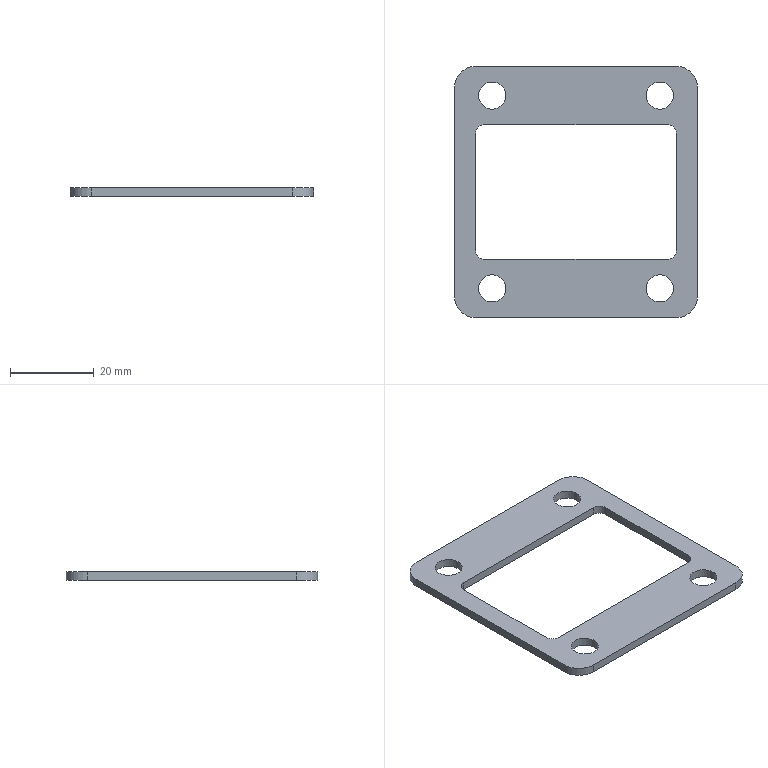Part | NX | features BREP 1 | 1 solid | 22 faces | box 58 x 60 x 2 mm | volume 3586 mm3 | cylinder 12 | plane 10 | commonest cylinder face diameters 4 x4 6.5 x4 10 x4
STEP:
#1=CARTESIAN_POINT('',(-23.25,23.,2.));
#2=VERTEX_POINT('',#1);
#3=CARTESIAN_POINT('',(-20.,23.,2.));
#4=DIRECTION('',(0.,0.,1.));
#5=DIRECTION('',(-1.,0.,0.));
#6=AXIS2_PLACEMENT_3D('',#3,#4,#5);
#7=CIRCLE('',#6,3.25);
#8=EDGE_CURVE('',#2,#2,#7,.T.);
#9=ORIENTED_EDGE('',*,*,#8,.T.);
#10=EDGE_LOOP('',(#9));
#11=FACE_BOUND('',#10,.T.);
#12=CARTESIAN_POINT('',(-23.25,23.,0.));
#13=VERTEX_POINT('',#12);
#14=CARTESIAN_POINT('',(-20.,23.,0.));
#15=DIRECTION('',(0.,0.,1.));
#16=DIRECTION('',(-1.,0.,0.));
#17=AXIS2_PLACEMENT_3D('',#14,#15,#16);
#18=CIRCLE('',#17,3.25);
#19=EDGE_CURVE('',#13,#13,#18,.T.);
#20=ORIENTED_EDGE('',*,*,#19,.F.);
#21=EDGE_LOOP('',(#20));
#22=FACE_BOUND('',#21,.T.);
#23=CARTESIAN_POINT('',(-20.,23.,0.));
#24=DIRECTION('',(0.,0.,1.));
#25=DIRECTION('',(1.,0.,0.));
#26=AXIS2_PLACEMENT_3D('',#23,#24,#25);
#27=CYLINDRICAL_SURFACE('',#26,3.25);
#28=ADVANCED_FACE('',(#11,#22),#27,.F.);
#29=CARTESIAN_POINT('',(-16.75,-23.,2.));
#30=VERTEX_POINT('',#29);
#31=CARTESIAN_POINT('',(-20.,-23.,2.));
#32=DIRECTION('',(0.,0.,1.));
#33=DIRECTION('',(1.,0.,0.));
#34=AXIS2_PLACEMENT_3D('',#31,#32,#33);
#35=CIRCLE('',#34,3.25);
#36=EDGE_CURVE('',#30,#30,#35,.T.);
#37=ORIENTED_EDGE('',*,*,#36,.T.);
#38=EDGE_LOOP('',(#37));
#39=FACE_BOUND('',#38,.T.);
#40=CARTESIAN_POINT('',(-16.75,-23.,0.));
#41=VERTEX_POINT('',#40);
#42=CARTESIAN_POINT('',(-20.,-23.,0.));
#43=DIRECTION('',(0.,0.,1.));
#44=DIRECTION('',(1.,0.,0.));
#45=AXIS2_PLACEMENT_3D('',#42,#43,#44);
#46=CIRCLE('',#45,3.25);
#47=EDGE_CURVE('',#41,#41,#46,.T.);
#48=ORIENTED_EDGE('',*,*,#47,.F.);
#49=EDGE_LOOP('',(#48));
#50=FACE_BOUND('',#49,.T.);
#51=CARTESIAN_POINT('',(-20.,-23.,0.));
#52=DIRECTION('',(0.,0.,1.));
#53=DIRECTION('',(1.,0.,0.));
#54=AXIS2_PLACEMENT_3D('',#51,#52,#53);
#55=CYLINDRICAL_SURFACE('',#54,3.25);
#56=ADVANCED_FACE('',(#39,#50),#55,.F.);
#57=CARTESIAN_POINT('',(16.75,-23.,2.));
#58=VERTEX_POINT('',#57);
#59=CARTESIAN_POINT('',(20.,-23.,2.));
#60=DIRECTION('',(0.,0.,1.));
#61=DIRECTION('',(-1.,0.,0.));
#62=AXIS2_PLACEMENT_3D('',#59,#60,#61);
#63=CIRCLE('',#62,3.25);
#64=EDGE_CURVE('',#58,#58,#63,.T.);
#65=ORIENTED_EDGE('',*,*,#64,.T.);
#66=EDGE_LOOP('',(#65));
#67=FACE_BOUND('',#66,.T.);
#68=CARTESIAN_POINT('',(16.75,-23.,0.));
#69=VERTEX_POINT('',#68);
#70=CARTESIAN_POINT('',(20.,-23.,0.));
#71=DIRECTION('',(0.,0.,1.));
#72=DIRECTION('',(-1.,0.,0.));
#73=AXIS2_PLACEMENT_3D('',#70,#71,#72);
#74=CIRCLE('',#73,3.25);
#75=EDGE_CURVE('',#69,#69,#74,.T.);
#76=ORIENTED_EDGE('',*,*,#75,.F.);
#77=EDGE_LOOP('',(#76));
#78=FACE_BOUND('',#77,.T.);
#79=CARTESIAN_POINT('',(20.,-23.,0.));
#80=DIRECTION('',(0.,0.,1.));
#81=DIRECTION('',(1.,0.,0.));
#82=AXIS2_PLACEMENT_3D('',#79,#80,#81);
#83=CYLINDRICAL_SURFACE('',#82,3.25);
#84=ADVANCED_FACE('',(#67,#78),#83,.F.);
#85=CARTESIAN_POINT('',(23.25,23.,2.));
#86=VERTEX_POINT('',#85);
#87=CARTESIAN_POINT('',(20.,23.,2.));
#88=DIRECTION('',(0.,0.,1.));
#89=DIRECTION('',(1.,0.,0.));
#90=AXIS2_PLACEMENT_3D('',#87,#88,#89);
#91=CIRCLE('',#90,3.25);
#92=EDGE_CURVE('',#86,#86,#91,.T.);
#93=ORIENTED_EDGE('',*,*,#92,.T.);
#94=EDGE_LOOP('',(#93));
#95=FACE_BOUND('',#94,.T.);
#96=CARTESIAN_POINT('',(23.25,23.,0.));
#97=VERTEX_POINT('',#96);
#98=CARTESIAN_POINT('',(20.,23.,0.));
#99=DIRECTION('',(0.,0.,1.));
#100=DIRECTION('',(1.,0.,0.));
#101=AXIS2_PLACEMENT_3D('',#98,#99,#100);
#102=CIRCLE('',#101,3.25);
#103=EDGE_CURVE('',#97,#97,#102,.T.);
#104=ORIENTED_EDGE('',*,*,#103,.F.);
#105=EDGE_LOOP('',(#104));
#106=FACE_BOUND('',#105,.T.);
#107=CARTESIAN_POINT('',(20.,23.,0.));
#108=DIRECTION('',(0.,0.,1.));
#109=DIRECTION('',(1.,0.,0.));
#110=AXIS2_PLACEMENT_3D('',#107,#108,#109);
#111=CYLINDRICAL_SURFACE('',#110,3.25);
#112=ADVANCED_FACE('',(#95,#106),#111,.F.);
#113=ORIENTED_EDGE('',*,*,#8,.F.);
#114=EDGE_LOOP('',(#113));
#115=FACE_BOUND('',#114,.T.);
#116=ORIENTED_EDGE('',*,*,#36,.F.);
#117=EDGE_LOOP('',(#116));
#118=FACE_BOUND('',#117,.T.);
#119=ORIENTED_EDGE('',*,*,#64,.F.);
#120=EDGE_LOOP('',(#119));
#121=FACE_BOUND('',#120,.T.);
#122=ORIENTED_EDGE('',*,*,#92,.F.);
#123=EDGE_LOOP('',(#122));
#124=FACE_BOUND('',#123,.T.);
#125=CARTESIAN_POINT('',(-29.,25.,2.));
#126=VERTEX_POINT('',#125);
#127=CARTESIAN_POINT('',(-29.,-25.,2.));
#128=VERTEX_POINT('',#127);
#129=CARTESIAN_POINT('',(-29.,30.,2.));
#130=DIRECTION('',(0.,-1.,0.));
#131=VECTOR('',#130,1000.);
#132=LINE('',#129,#131);
#133=EDGE_CURVE('',#126,#128,#132,.T.);
#134=ORIENTED_EDGE('',*,*,#133,.T.);
#135=CARTESIAN_POINT('',(-24.,-30.,2.));
#136=VERTEX_POINT('',#135);
#137=CARTESIAN_POINT('',(-24.,-25.,2.));
#138=DIRECTION('',(0.,0.,1.));
#139=DIRECTION('',(1.,0.,0.));
#140=AXIS2_PLACEMENT_3D('',#137,#138,#139);
#141=CIRCLE('',#140,5.);
#142=EDGE_CURVE('',#128,#136,#141,.T.);
#143=ORIENTED_EDGE('',*,*,#142,.T.);
#144=CARTESIAN_POINT('',(24.,-30.,2.));
#145=VERTEX_POINT('',#144);
#146=CARTESIAN_POINT('',(-29.,-30.,2.));
#147=DIRECTION('',(1.,0.,0.));
#148=VECTOR('',#147,1000.);
#149=LINE('',#146,#148);
#150=EDGE_CURVE('',#136,#145,#149,.T.);
#151=ORIENTED_EDGE('',*,*,#150,.T.);
#152=CARTESIAN_POINT('',(29.,-25.,2.));
#153=VERTEX_POINT('',#152);
#154=CARTESIAN_POINT('',(24.,-25.,2.));
#155=DIRECTION('',(0.,0.,1.));
#156=DIRECTION('',(1.,0.,0.));
#157=AXIS2_PLACEMENT_3D('',#154,#155,#156);
#158=CIRCLE('',#157,5.);
#159=EDGE_CURVE('',#145,#153,#158,.T.);
#160=ORIENTED_EDGE('',*,*,#159,.T.);
#161=CARTESIAN_POINT('',(29.,25.,2.));
#162=VERTEX_POINT('',#161);
#163=CARTESIAN_POINT('',(29.,30.,2.));
#164=DIRECTION('',(0.,1.,0.));
#165=VECTOR('',#164,1000.);
#166=LINE('',#163,#165);
#167=EDGE_CURVE('',#153,#162,#166,.T.);
#168=ORIENTED_EDGE('',*,*,#167,.T.);
#169=CARTESIAN_POINT('',(24.,30.,2.));
#170=VERTEX_POINT('',#169);
#171=CARTESIAN_POINT('',(24.,25.,2.));
#172=DIRECTION('',(0.,0.,1.));
#173=DIRECTION('',(1.,0.,0.));
#174=AXIS2_PLACEMENT_3D('',#171,#172,#173);
#175=CIRCLE('',#174,5.);
#176=EDGE_CURVE('',#162,#170,#175,.T.);
#177=ORIENTED_EDGE('',*,*,#176,.T.);
#178=CARTESIAN_POINT('',(-24.,30.,2.));
#179=VERTEX_POINT('',#178);
#180=CARTESIAN_POINT('',(-29.,30.,2.));
#181=DIRECTION('',(-1.,0.,0.));
#182=VECTOR('',#181,1000.);
#183=LINE('',#180,#182);
#184=EDGE_CURVE('',#170,#179,#183,.T.);
#185=ORIENTED_EDGE('',*,*,#184,.T.);
#186=CARTESIAN_POINT('',(-24.,25.,2.));
#187=DIRECTION('',(0.,0.,1.));
#188=DIRECTION('',(1.,0.,0.));
#189=AXIS2_PLACEMENT_3D('',#186,#187,#188);
#190=CIRCLE('',#189,5.);
#191=EDGE_CURVE('',#179,#126,#190,.T.);
#192=ORIENTED_EDGE('',*,*,#191,.T.);
#193=EDGE_LOOP('',(#134,#143,#151,#160,#168,#177,#185,#192));
#194=FACE_BOUND('',#193,.T.);
#195=CARTESIAN_POINT('',(22.,16.,2.));
#196=VERTEX_POINT('',#195);
#197=CARTESIAN_POINT('',(-22.,16.,2.));
#198=VERTEX_POINT('',#197);
#199=CARTESIAN_POINT('',(-24.,16.,2.));
#200=DIRECTION('',(-1.,0.,0.));
#201=VECTOR('',#200,1000.);
#202=LINE('',#199,#201);
#203=EDGE_CURVE('',#196,#198,#202,.T.);
#204=ORIENTED_EDGE('',*,*,#203,.F.);
#205=CARTESIAN_POINT('',(24.,14.,2.));
#206=VERTEX_POINT('',#205);
#207=CARTESIAN_POINT('',(22.,14.,2.));
#208=DIRECTION('',(0.,0.,-1.));
#209=DIRECTION('',(1.,0.,0.));
#210=AXIS2_PLACEMENT_3D('',#207,#208,#209);
#211=CIRCLE('',#210,2.);
#212=EDGE_CURVE('',#196,#206,#211,.T.);
#213=ORIENTED_EDGE('',*,*,#212,.T.);
#214=CARTESIAN_POINT('',(24.,-14.,2.));
#215=VERTEX_POINT('',#214);
#216=CARTESIAN_POINT('',(24.,16.,2.));
#217=DIRECTION('',(0.,1.,0.));
#218=VECTOR('',#217,1000.);
#219=LINE('',#216,#218);
#220=EDGE_CURVE('',#215,#206,#219,.T.);
#221=ORIENTED_EDGE('',*,*,#220,.F.);
#222=CARTESIAN_POINT('',(22.,-16.,2.));
#223=VERTEX_POINT('',#222);
#224=CARTESIAN_POINT('',(22.,-14.,2.));
#225=DIRECTION('',(0.,0.,-1.));
#226=DIRECTION('',(1.,0.,0.));
#227=AXIS2_PLACEMENT_3D('',#224,#225,#226);
#228=CIRCLE('',#227,2.);
#229=EDGE_CURVE('',#215,#223,#228,.T.);
#230=ORIENTED_EDGE('',*,*,#229,.T.);
#231=CARTESIAN_POINT('',(-22.,-16.,2.));
#232=VERTEX_POINT('',#231);
#233=CARTESIAN_POINT('',(-24.,-16.,2.));
#234=DIRECTION('',(1.,0.,0.));
#235=VECTOR('',#234,1000.);
#236=LINE('',#233,#235);
#237=EDGE_CURVE('',#232,#223,#236,.T.);
#238=ORIENTED_EDGE('',*,*,#237,.F.);
#239=CARTESIAN_POINT('',(-24.,-14.,2.));
#240=VERTEX_POINT('',#239);
#241=CARTESIAN_POINT('',(-22.,-14.,2.));
#242=DIRECTION('',(0.,0.,-1.));
#243=DIRECTION('',(1.,0.,0.));
#244=AXIS2_PLACEMENT_3D('',#241,#242,#243);
#245=CIRCLE('',#244,2.);
#246=EDGE_CURVE('',#232,#240,#245,.T.);
#247=ORIENTED_EDGE('',*,*,#246,.T.);
#248=CARTESIAN_POINT('',(-24.,14.,2.));
#249=VERTEX_POINT('',#248);
#250=CARTESIAN_POINT('',(-24.,16.,2.));
#251=DIRECTION('',(0.,-1.,0.));
#252=VECTOR('',#251,1000.);
#253=LINE('',#250,#252);
#254=EDGE_CURVE('',#249,#240,#253,.T.);
#255=ORIENTED_EDGE('',*,*,#254,.F.);
#256=CARTESIAN_POINT('',(-22.,14.,2.));
#257=DIRECTION('',(0.,0.,-1.));
#258=DIRECTION('',(1.,0.,0.));
#259=AXIS2_PLACEMENT_3D('',#256,#257,#258);
#260=CIRCLE('',#259,2.);
#261=EDGE_CURVE('',#249,#198,#260,.T.);
#262=ORIENTED_EDGE('',*,*,#261,.T.);
#263=EDGE_LOOP('',(#204,#213,#221,#230,#238,#247,#255,#262));
#264=FACE_BOUND('',#263,.T.);
#265=CARTESIAN_POINT('',(0.,0.,2.));
#266=DIRECTION('',(0.,0.,1.));
#267=DIRECTION('',(1.,0.,0.));
#268=AXIS2_PLACEMENT_3D('',#265,#266,#267);
#269=PLANE('',#268);
#270=ADVANCED_FACE('',(#115,#118,#121,#124,#194,#264),#269,.T.);
#271=ORIENTED_EDGE('',*,*,#19,.T.);
#272=EDGE_LOOP('',(#271));
#273=FACE_BOUND('',#272,.T.);
#274=ORIENTED_EDGE('',*,*,#47,.T.);
#275=EDGE_LOOP('',(#274));
#276=FACE_BOUND('',#275,.T.);
#277=ORIENTED_EDGE('',*,*,#75,.T.);
#278=EDGE_LOOP('',(#277));
#279=FACE_BOUND('',#278,.T.);
#280=ORIENTED_EDGE('',*,*,#103,.T.);
#281=EDGE_LOOP('',(#280));
#282=FACE_BOUND('',#281,.T.);
#283=CARTESIAN_POINT('',(-24.,-30.,0.));
#284=VERTEX_POINT('',#283);
#285=CARTESIAN_POINT('',(24.,-30.,0.));
#286=VERTEX_POINT('',#285);
#287=CARTESIAN_POINT('',(-29.,-30.,0.));
#288=DIRECTION('',(1.,0.,0.));
#289=VECTOR('',#288,1000.);
#290=LINE('',#287,#289);
#291=EDGE_CURVE('',#284,#286,#290,.T.);
#292=ORIENTED_EDGE('',*,*,#291,.F.);
#293=CARTESIAN_POINT('',(-29.,-25.,0.));
#294=VERTEX_POINT('',#293);
#295=CARTESIAN_POINT('',(-24.,-25.,0.));
#296=DIRECTION('',(0.,0.,-1.));
#297=DIRECTION('',(1.,0.,0.));
#298=AXIS2_PLACEMENT_3D('',#295,#296,#297);
#299=CIRCLE('',#298,5.);
#300=EDGE_CURVE('',#284,#294,#299,.T.);
#301=ORIENTED_EDGE('',*,*,#300,.T.);
#302=CARTESIAN_POINT('',(-29.,25.,0.));
#303=VERTEX_POINT('',#302);
#304=CARTESIAN_POINT('',(-29.,30.,0.));
#305=DIRECTION('',(0.,-1.,0.));
#306=VECTOR('',#305,1000.);
#307=LINE('',#304,#306);
#308=EDGE_CURVE('',#303,#294,#307,.T.);
#309=ORIENTED_EDGE('',*,*,#308,.F.);
#310=CARTESIAN_POINT('',(-24.,30.,0.));
#311=VERTEX_POINT('',#310);
#312=CARTESIAN_POINT('',(-24.,25.,0.));
#313=DIRECTION('',(0.,0.,-1.));
#314=DIRECTION('',(1.,0.,0.));
#315=AXIS2_PLACEMENT_3D('',#312,#313,#314);
#316=CIRCLE('',#315,5.);
#317=EDGE_CURVE('',#303,#311,#316,.T.);
#318=ORIENTED_EDGE('',*,*,#317,.T.);
#319=CARTESIAN_POINT('',(24.,30.,0.));
#320=VERTEX_POINT('',#319);
#321=CARTESIAN_POINT('',(-29.,30.,0.));
#322=DIRECTION('',(-1.,0.,0.));
#323=VECTOR('',#322,1000.);
#324=LINE('',#321,#323);
#325=EDGE_CURVE('',#320,#311,#324,.T.);
#326=ORIENTED_EDGE('',*,*,#325,.F.);
#327=CARTESIAN_POINT('',(29.,25.,0.));
#328=VERTEX_POINT('',#327);
#329=CARTESIAN_POINT('',(24.,25.,0.));
#330=DIRECTION('',(0.,0.,-1.));
#331=DIRECTION('',(1.,0.,0.));
#332=AXIS2_PLACEMENT_3D('',#329,#330,#331);
#333=CIRCLE('',#332,5.);
#334=EDGE_CURVE('',#320,#328,#333,.T.);
#335=ORIENTED_EDGE('',*,*,#334,.T.);
#336=CARTESIAN_POINT('',(29.,-25.,0.));
#337=VERTEX_POINT('',#336);
#338=CARTESIAN_POINT('',(29.,30.,0.));
#339=DIRECTION('',(0.,1.,0.));
#340=VECTOR('',#339,1000.);
#341=LINE('',#338,#340);
#342=EDGE_CURVE('',#337,#328,#341,.T.);
#343=ORIENTED_EDGE('',*,*,#342,.F.);
#344=CARTESIAN_POINT('',(24.,-25.,0.));
#345=DIRECTION('',(0.,0.,-1.));
#346=DIRECTION('',(1.,0.,0.));
#347=AXIS2_PLACEMENT_3D('',#344,#345,#346);
#348=CIRCLE('',#347,5.);
#349=EDGE_CURVE('',#337,#286,#348,.T.);
#350=ORIENTED_EDGE('',*,*,#349,.T.);
#351=EDGE_LOOP('',(#292,#301,#309,#318,#326,#335,#343,#350));
#352=FACE_BOUND('',#351,.T.);
#353=CARTESIAN_POINT('',(-22.,-16.,0.));
#354=VERTEX_POINT('',#353);
#355=CARTESIAN_POINT('',(22.,-16.,0.));
#356=VERTEX_POINT('',#355);
#357=CARTESIAN_POINT('',(-24.,-16.,0.));
#358=DIRECTION('',(1.,0.,0.));
#359=VECTOR('',#358,1000.);
#360=LINE('',#357,#359);
#361=EDGE_CURVE('',#354,#356,#360,.T.);
#362=ORIENTED_EDGE('',*,*,#361,.T.);
#363=CARTESIAN_POINT('',(24.,-14.,0.));
#364=VERTEX_POINT('',#363);
#365=CARTESIAN_POINT('',(22.,-14.,0.));
#366=DIRECTION('',(0.,0.,1.));
#367=DIRECTION('',(1.,0.,0.));
#368=AXIS2_PLACEMENT_3D('',#365,#366,#367);
#369=CIRCLE('',#368,2.);
#370=EDGE_CURVE('',#356,#364,#369,.T.);
#371=ORIENTED_EDGE('',*,*,#370,.T.);
#372=CARTESIAN_POINT('',(24.,14.,0.));
#373=VERTEX_POINT('',#372);
#374=CARTESIAN_POINT('',(24.,16.,0.));
#375=DIRECTION('',(0.,1.,0.));
#376=VECTOR('',#375,1000.);
#377=LINE('',#374,#376);
#378=EDGE_CURVE('',#364,#373,#377,.T.);
#379=ORIENTED_EDGE('',*,*,#378,.T.);
#380=CARTESIAN_POINT('',(22.,16.,0.));
#381=VERTEX_POINT('',#380);
#382=CARTESIAN_POINT('',(22.,14.,0.));
#383=DIRECTION('',(0.,0.,1.));
#384=DIRECTION('',(1.,0.,0.));
#385=AXIS2_PLACEMENT_3D('',#382,#383,#384);
#386=CIRCLE('',#385,2.);
#387=EDGE_CURVE('',#373,#381,#386,.T.);
#388=ORIENTED_EDGE('',*,*,#387,.T.);
#389=CARTESIAN_POINT('',(-22.,16.,0.));
#390=VERTEX_POINT('',#389);
#391=CARTESIAN_POINT('',(-24.,16.,0.));
#392=DIRECTION('',(-1.,0.,0.));
#393=VECTOR('',#392,1000.);
#394=LINE('',#391,#393);
#395=EDGE_CURVE('',#381,#390,#394,.T.);
#396=ORIENTED_EDGE('',*,*,#395,.T.);
#397=CARTESIAN_POINT('',(-24.,14.,0.));
#398=VERTEX_POINT('',#397);
#399=CARTESIAN_POINT('',(-22.,14.,0.));
#400=DIRECTION('',(0.,0.,1.));
#401=DIRECTION('',(1.,0.,0.));
#402=AXIS2_PLACEMENT_3D('',#399,#400,#401);
#403=CIRCLE('',#402,2.);
#404=EDGE_CURVE('',#390,#398,#403,.T.);
#405=ORIENTED_EDGE('',*,*,#404,.T.);
#406=CARTESIAN_POINT('',(-24.,-14.,0.));
#407=VERTEX_POINT('',#406);
#408=CARTESIAN_POINT('',(-24.,16.,0.));
#409=DIRECTION('',(0.,-1.,0.));
#410=VECTOR('',#409,1000.);
#411=LINE('',#408,#410);
#412=EDGE_CURVE('',#398,#407,#411,.T.);
#413=ORIENTED_EDGE('',*,*,#412,.T.);
#414=CARTESIAN_POINT('',(-22.,-14.,0.));
#415=DIRECTION('',(0.,0.,1.));
#416=DIRECTION('',(1.,0.,0.));
#417=AXIS2_PLACEMENT_3D('',#414,#415,#416);
#418=CIRCLE('',#417,2.);
#419=EDGE_CURVE('',#407,#354,#418,.T.);
#420=ORIENTED_EDGE('',*,*,#419,.T.);
#421=EDGE_LOOP('',(#362,#371,#379,#388,#396,#405,#413,#420));
#422=FACE_BOUND('',#421,.T.);
#423=CARTESIAN_POINT('',(0.,0.,0.));
#424=DIRECTION('',(0.,0.,1.));
#425=DIRECTION('',(1.,0.,0.));
#426=AXIS2_PLACEMENT_3D('',#423,#424,#425);
#427=PLANE('',#426);
#428=ADVANCED_FACE('',(#273,#276,#279,#282,#352,#422),#427,.F.);
#429=ORIENTED_EDGE('',*,*,#167,.F.);
#430=CARTESIAN_POINT('',(29.,-25.,2.));
#431=DIRECTION('',(0.,0.,-1.));
#432=VECTOR('',#431,1000.);
#433=LINE('',#430,#432);
#434=EDGE_CURVE('',#153,#337,#433,.T.);
#435=ORIENTED_EDGE('',*,*,#434,.T.);
#436=ORIENTED_EDGE('',*,*,#342,.T.);
#437=CARTESIAN_POINT('',(29.,25.,2.));
#438=DIRECTION('',(0.,0.,1.));
#439=VECTOR('',#438,1000.);
#440=LINE('',#437,#439);
#441=EDGE_CURVE('',#328,#162,#440,.T.);
#442=ORIENTED_EDGE('',*,*,#441,.T.);
#443=EDGE_LOOP('',(#429,#435,#436,#442));
#444=FACE_BOUND('',#443,.T.);
#445=CARTESIAN_POINT('',(29.,30.,2.));
#446=DIRECTION('',(-1.,0.,0.));
#447=DIRECTION('',(0.,-1.,0.));
#448=AXIS2_PLACEMENT_3D('',#445,#446,#447);
#449=PLANE('',#448);
#450=ADVANCED_FACE('',(#444),#449,.F.);
#451=ORIENTED_EDGE('',*,*,#184,.F.);
#452=CARTESIAN_POINT('',(24.,30.,2.));
#453=DIRECTION('',(0.,0.,-1.));
#454=VECTOR('',#453,1000.);
#455=LINE('',#452,#454);
#456=EDGE_CURVE('',#170,#320,#455,.T.);
#457=ORIENTED_EDGE('',*,*,#456,.T.);
#458=ORIENTED_EDGE('',*,*,#325,.T.);
#459=CARTESIAN_POINT('',(-24.,30.,2.));
#460=DIRECTION('',(0.,0.,1.));
#461=VECTOR('',#460,1000.);
#462=LINE('',#459,#461);
#463=EDGE_CURVE('',#311,#179,#462,.T.);
#464=ORIENTED_EDGE('',*,*,#463,.T.);
#465=EDGE_LOOP('',(#451,#457,#458,#464));
#466=FACE_BOUND('',#465,.T.);
#467=CARTESIAN_POINT('',(-29.,30.,2.));
#468=DIRECTION('',(0.,-1.,0.));
#469=DIRECTION('',(0.,0.,-1.));
#470=AXIS2_PLACEMENT_3D('',#467,#468,#469);
#471=PLANE('',#470);
#472=ADVANCED_FACE('',(#466),#471,.F.);
#473=ORIENTED_EDGE('',*,*,#308,.T.);
#474=CARTESIAN_POINT('',(-29.,-25.,2.));
#475=DIRECTION('',(0.,0.,1.));
#476=VECTOR('',#475,1000.);
#477=LINE('',#474,#476);
#478=EDGE_CURVE('',#294,#128,#477,.T.);
#479=ORIENTED_EDGE('',*,*,#478,.T.);
#480=ORIENTED_EDGE('',*,*,#133,.F.);
#481=CARTESIAN_POINT('',(-29.,25.,2.));
#482=DIRECTION('',(0.,0.,-1.));
#483=VECTOR('',#482,1000.);
#484=LINE('',#481,#483);
#485=EDGE_CURVE('',#126,#303,#484,.T.);
#486=ORIENTED_EDGE('',*,*,#485,.T.);
#487=EDGE_LOOP('',(#473,#479,#480,#486));
#488=FACE_BOUND('',#487,.T.);
#489=CARTESIAN_POINT('',(-29.,30.,2.));
#490=DIRECTION('',(1.,0.,0.));
#491=DIRECTION('',(0.,1.,0.));
#492=AXIS2_PLACEMENT_3D('',#489,#490,#491);
#493=PLANE('',#492);
#494=ADVANCED_FACE('',(#488),#493,.F.);
#495=ORIENTED_EDGE('',*,*,#150,.F.);
#496=CARTESIAN_POINT('',(-24.,-30.,2.));
#497=DIRECTION('',(0.,0.,-1.));
#498=VECTOR('',#497,1000.);
#499=LINE('',#496,#498);
#500=EDGE_CURVE('',#136,#284,#499,.T.);
#501=ORIENTED_EDGE('',*,*,#500,.T.);
#502=ORIENTED_EDGE('',*,*,#291,.T.);
#503=CARTESIAN_POINT('',(24.,-30.,2.));
#504=DIRECTION('',(0.,0.,1.));
#505=VECTOR('',#504,1000.);
#506=LINE('',#503,#505);
#507=EDGE_CURVE('',#286,#145,#506,.T.);
#508=ORIENTED_EDGE('',*,*,#507,.T.);
#509=EDGE_LOOP('',(#495,#501,#502,#508));
#510=FACE_BOUND('',#509,.T.);
#511=CARTESIAN_POINT('',(-29.,-30.,2.));
#512=DIRECTION('',(0.,1.,0.));
#513=DIRECTION('',(0.,0.,1.));
#514=AXIS2_PLACEMENT_3D('',#511,#512,#513);
#515=PLANE('',#514);
#516=ADVANCED_FACE('',(#510),#515,.F.);
#517=ORIENTED_EDGE('',*,*,#220,.T.);
#518=CARTESIAN_POINT('',(24.,14.,0.));
#519=DIRECTION('',(0.,0.,-1.));
#520=VECTOR('',#519,1000.);
#521=LINE('',#518,#520);
#522=EDGE_CURVE('',#206,#373,#521,.T.);
#523=ORIENTED_EDGE('',*,*,#522,.T.);
#524=ORIENTED_EDGE('',*,*,#378,.F.);
#525=CARTESIAN_POINT('',(24.,-14.,2.));
#526=DIRECTION('',(0.,0.,1.));
#527=VECTOR('',#526,1000.);
#528=LINE('',#525,#527);
#529=EDGE_CURVE('',#364,#215,#528,.T.);
#530=ORIENTED_EDGE('',*,*,#529,.T.);
#531=EDGE_LOOP('',(#517,#523,#524,#530));
#532=FACE_BOUND('',#531,.T.);
#533=CARTESIAN_POINT('',(24.,16.,2.));
#534=DIRECTION('',(-1.,0.,0.));
#535=DIRECTION('',(0.,-1.,0.));
#536=AXIS2_PLACEMENT_3D('',#533,#534,#535);
#537=PLANE('',#536);
#538=ADVANCED_FACE('',(#532),#537,.T.);
#539=ORIENTED_EDGE('',*,*,#203,.T.);
#540=CARTESIAN_POINT('',(-22.,16.,0.));
#541=DIRECTION('',(0.,0.,-1.));
#542=VECTOR('',#541,1000.);
#543=LINE('',#540,#542);
#544=EDGE_CURVE('',#198,#390,#543,.T.);
#545=ORIENTED_EDGE('',*,*,#544,.T.);
#546=ORIENTED_EDGE('',*,*,#395,.F.);
#547=CARTESIAN_POINT('',(22.,16.,2.));
#548=DIRECTION('',(0.,0.,1.));
#549=VECTOR('',#548,1000.);
#550=LINE('',#547,#549);
#551=EDGE_CURVE('',#381,#196,#550,.T.);
#552=ORIENTED_EDGE('',*,*,#551,.T.);
#553=EDGE_LOOP('',(#539,#545,#546,#552));
#554=FACE_BOUND('',#553,.T.);
#555=CARTESIAN_POINT('',(-24.,16.,2.));
#556=DIRECTION('',(0.,-1.,0.));
#557=DIRECTION('',(0.,0.,-1.));
#558=AXIS2_PLACEMENT_3D('',#555,#556,#557);
#559=PLANE('',#558);
#560=ADVANCED_FACE('',(#554),#559,.T.);
#561=ORIENTED_EDGE('',*,*,#254,.T.);
#562=CARTESIAN_POINT('',(-24.,-14.,0.));
#563=DIRECTION('',(0.,0.,-1.));
#564=VECTOR('',#563,1000.);
#565=LINE('',#562,#564);
#566=EDGE_CURVE('',#240,#407,#565,.T.);
#567=ORIENTED_EDGE('',*,*,#566,.T.);
#568=ORIENTED_EDGE('',*,*,#412,.F.);
#569=CARTESIAN_POINT('',(-24.,14.,2.));
#570=DIRECTION('',(0.,0.,1.));
#571=VECTOR('',#570,1000.);
#572=LINE('',#569,#571);
#573=EDGE_CURVE('',#398,#249,#572,.T.);
#574=ORIENTED_EDGE('',*,*,#573,.T.);
#575=EDGE_LOOP('',(#561,#567,#568,#574));
#576=FACE_BOUND('',#575,.T.);
#577=CARTESIAN_POINT('',(-24.,16.,2.));
#578=DIRECTION('',(1.,0.,0.));
#579=DIRECTION('',(0.,1.,0.));
#580=AXIS2_PLACEMENT_3D('',#577,#578,#579);
#581=PLANE('',#580);
#582=ADVANCED_FACE('',(#576),#581,.T.);
#583=ORIENTED_EDGE('',*,*,#361,.F.);
#584=CARTESIAN_POINT('',(-22.,-16.,2.));
#585=DIRECTION('',(0.,0.,1.));
#586=VECTOR('',#585,1000.);
#587=LINE('',#584,#586);
#588=EDGE_CURVE('',#354,#232,#587,.T.);
#589=ORIENTED_EDGE('',*,*,#588,.T.);
#590=ORIENTED_EDGE('',*,*,#237,.T.);
#591=CARTESIAN_POINT('',(22.,-16.,0.));
#592=DIRECTION('',(0.,0.,-1.));
#593=VECTOR('',#592,1000.);
#594=LINE('',#591,#593);
#595=EDGE_CURVE('',#223,#356,#594,.T.);
#596=ORIENTED_EDGE('',*,*,#595,.T.);
#597=EDGE_LOOP('',(#583,#589,#590,#596));
#598=FACE_BOUND('',#597,.T.);
#599=CARTESIAN_POINT('',(-24.,-16.,2.));
#600=DIRECTION('',(0.,1.,0.));
#601=DIRECTION('',(0.,0.,1.));
#602=AXIS2_PLACEMENT_3D('',#599,#600,#601);
#603=PLANE('',#602);
#604=ADVANCED_FACE('',(#598),#603,.T.);
#605=ORIENTED_EDGE('',*,*,#142,.F.);
#606=ORIENTED_EDGE('',*,*,#478,.F.);
#607=ORIENTED_EDGE('',*,*,#300,.F.);
#608=ORIENTED_EDGE('',*,*,#500,.F.);
#609=EDGE_LOOP('',(#605,#606,#607,#608));
#610=FACE_BOUND('',#609,.T.);
#611=CARTESIAN_POINT('',(-24.,-25.,2.));
#612=DIRECTION('',(0.,0.,-1.));
#613=DIRECTION('',(-1.,0.,0.));
#614=AXIS2_PLACEMENT_3D('',#611,#612,#613);
#615=CYLINDRICAL_SURFACE('',#614,5.);
#616=ADVANCED_FACE('',(#610),#615,.T.);
#617=ORIENTED_EDGE('',*,*,#159,.F.);
#618=ORIENTED_EDGE('',*,*,#507,.F.);
#619=ORIENTED_EDGE('',*,*,#349,.F.);
#620=ORIENTED_EDGE('',*,*,#434,.F.);
#621=EDGE_LOOP('',(#617,#618,#619,#620));
#622=FACE_BOUND('',#621,.T.);
#623=CARTESIAN_POINT('',(24.,-25.,2.));
#624=DIRECTION('',(0.,0.,-1.));
#625=DIRECTION('',(-1.,0.,0.));
#626=AXIS2_PLACEMENT_3D('',#623,#624,#625);
#627=CYLINDRICAL_SURFACE('',#626,5.);
#628=ADVANCED_FACE('',(#622),#627,.T.);
#629=ORIENTED_EDGE('',*,*,#176,.F.);
#630=ORIENTED_EDGE('',*,*,#441,.F.);
#631=ORIENTED_EDGE('',*,*,#334,.F.);
#632=ORIENTED_EDGE('',*,*,#456,.F.);
#633=EDGE_LOOP('',(#629,#630,#631,#632));
#634=FACE_BOUND('',#633,.T.);
#635=CARTESIAN_POINT('',(24.,25.,2.));
#636=DIRECTION('',(0.,0.,-1.));
#637=DIRECTION('',(-1.,0.,0.));
#638=AXIS2_PLACEMENT_3D('',#635,#636,#637);
#639=CYLINDRICAL_SURFACE('',#638,5.);
#640=ADVANCED_FACE('',(#634),#639,.T.);
#641=ORIENTED_EDGE('',*,*,#191,.F.);
#642=ORIENTED_EDGE('',*,*,#463,.F.);
#643=ORIENTED_EDGE('',*,*,#317,.F.);
#644=ORIENTED_EDGE('',*,*,#485,.F.);
#645=EDGE_LOOP('',(#641,#642,#643,#644));
#646=FACE_BOUND('',#645,.T.);
#647=CARTESIAN_POINT('',(-24.,25.,2.));
#648=DIRECTION('',(0.,0.,-1.));
#649=DIRECTION('',(-1.,0.,0.));
#650=AXIS2_PLACEMENT_3D('',#647,#648,#649);
#651=CYLINDRICAL_SURFACE('',#650,5.);
#652=ADVANCED_FACE('',(#646),#651,.T.);
#653=ORIENTED_EDGE('',*,*,#246,.F.);
#654=ORIENTED_EDGE('',*,*,#588,.F.);
#655=ORIENTED_EDGE('',*,*,#419,.F.);
#656=ORIENTED_EDGE('',*,*,#566,.F.);
#657=EDGE_LOOP('',(#653,#654,#655,#656));
#658=FACE_BOUND('',#657,.T.);
#659=CARTESIAN_POINT('',(-22.,-14.,2.));
#660=DIRECTION('',(0.,0.,1.));
#661=DIRECTION('',(1.,0.,0.));
#662=AXIS2_PLACEMENT_3D('',#659,#660,#661);
#663=CYLINDRICAL_SURFACE('',#662,2.);
#664=ADVANCED_FACE('',(#658),#663,.F.);
#665=ORIENTED_EDGE('',*,*,#261,.F.);
#666=ORIENTED_EDGE('',*,*,#573,.F.);
#667=ORIENTED_EDGE('',*,*,#404,.F.);
#668=ORIENTED_EDGE('',*,*,#544,.F.);
#669=EDGE_LOOP('',(#665,#666,#667,#668));
#670=FACE_BOUND('',#669,.T.);
#671=CARTESIAN_POINT('',(-22.,14.,2.));
#672=DIRECTION('',(0.,0.,1.));
#673=DIRECTION('',(1.,0.,0.));
#674=AXIS2_PLACEMENT_3D('',#671,#672,#673);
#675=CYLINDRICAL_SURFACE('',#674,2.);
#676=ADVANCED_FACE('',(#670),#675,.F.);
#677=ORIENTED_EDGE('',*,*,#212,.F.);
#678=ORIENTED_EDGE('',*,*,#551,.F.);
#679=ORIENTED_EDGE('',*,*,#387,.F.);
#680=ORIENTED_EDGE('',*,*,#522,.F.);
#681=EDGE_LOOP('',(#677,#678,#679,#680));
#682=FACE_BOUND('',#681,.T.);
#683=CARTESIAN_POINT('',(22.,14.,2.));
#684=DIRECTION('',(0.,0.,1.));
#685=DIRECTION('',(1.,0.,0.));
#686=AXIS2_PLACEMENT_3D('',#683,#684,#685);
#687=CYLINDRICAL_SURFACE('',#686,2.);
#688=ADVANCED_FACE('',(#682),#687,.F.);
#689=ORIENTED_EDGE('',*,*,#229,.F.);
#690=ORIENTED_EDGE('',*,*,#529,.F.);
#691=ORIENTED_EDGE('',*,*,#370,.F.);
#692=ORIENTED_EDGE('',*,*,#595,.F.);
#693=EDGE_LOOP('',(#689,#690,#691,#692));
#694=FACE_BOUND('',#693,.T.);
#695=CARTESIAN_POINT('',(22.,-14.,2.));
#696=DIRECTION('',(0.,0.,1.));
#697=DIRECTION('',(1.,0.,0.));
#698=AXIS2_PLACEMENT_3D('',#695,#696,#697);
#699=CYLINDRICAL_SURFACE('',#698,2.);
#700=ADVANCED_FACE('',(#694),#699,.F.);
#701=CLOSED_SHELL('',(#28,#56,#84,#112,#270,#428,#450,#472,#494,#516,#538,#560,#582,#604,#616,#628,#640,#652,#664,#676,#688,#700));
#702=MANIFOLD_SOLID_BREP('',#701);
#703=(LENGTH_UNIT()NAMED_UNIT(*)SI_UNIT(.MILLI.,.METRE.));
#704=UNCERTAINTY_MEASURE_WITH_UNIT(LENGTH_MEASURE(0.00001),#703,'','');
#705=(NAMED_UNIT(*)PLANE_ANGLE_UNIT()SI_UNIT($,.RADIAN.));
#706=(NAMED_UNIT(*)SI_UNIT($,.STERADIAN.)SOLID_ANGLE_UNIT());
#707=(GEOMETRIC_REPRESENTATION_CONTEXT(3)GLOBAL_UNCERTAINTY_ASSIGNED_CONTEXT((#704))GLOBAL_UNIT_ASSIGNED_CONTEXT((#703,#705,#706))REPRESENTATION_CONTEXT('',''));
#708=ADVANCED_BREP_SHAPE_REPRESENTATION('',(#702),#707);